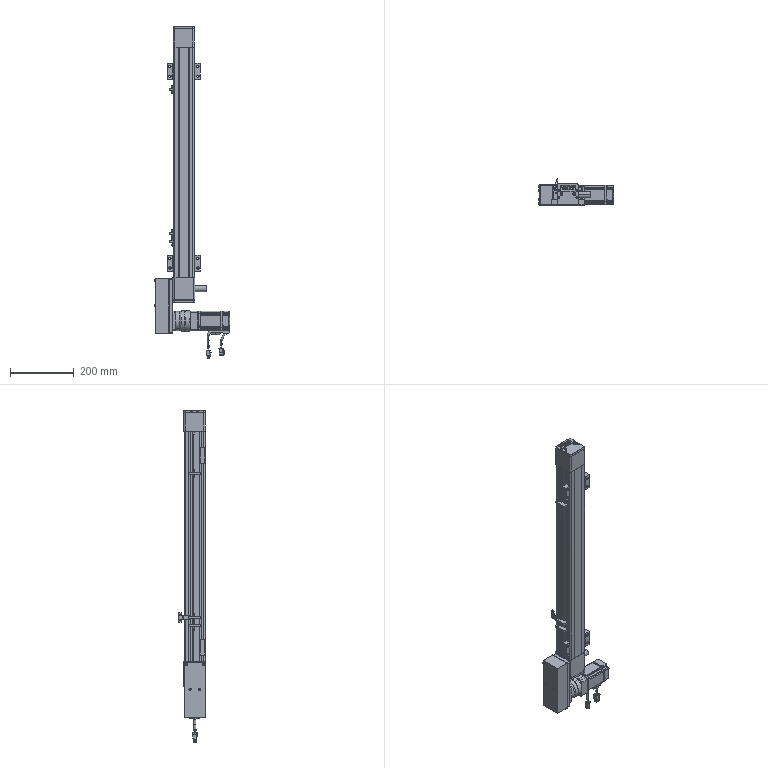Part | SolidWorks | 19 solids | 2674 faces | box 236 x 83 x 1039 mm | volume 3946589 mm3 | plane 1378 | cylinder 774 | cone 408 | spline 64 | torus 44 | sphere 6 | commonest cylinder face diameters 6 x81 5.5 x72 0.6 x59 8 x57 4 x49 4.5 x48